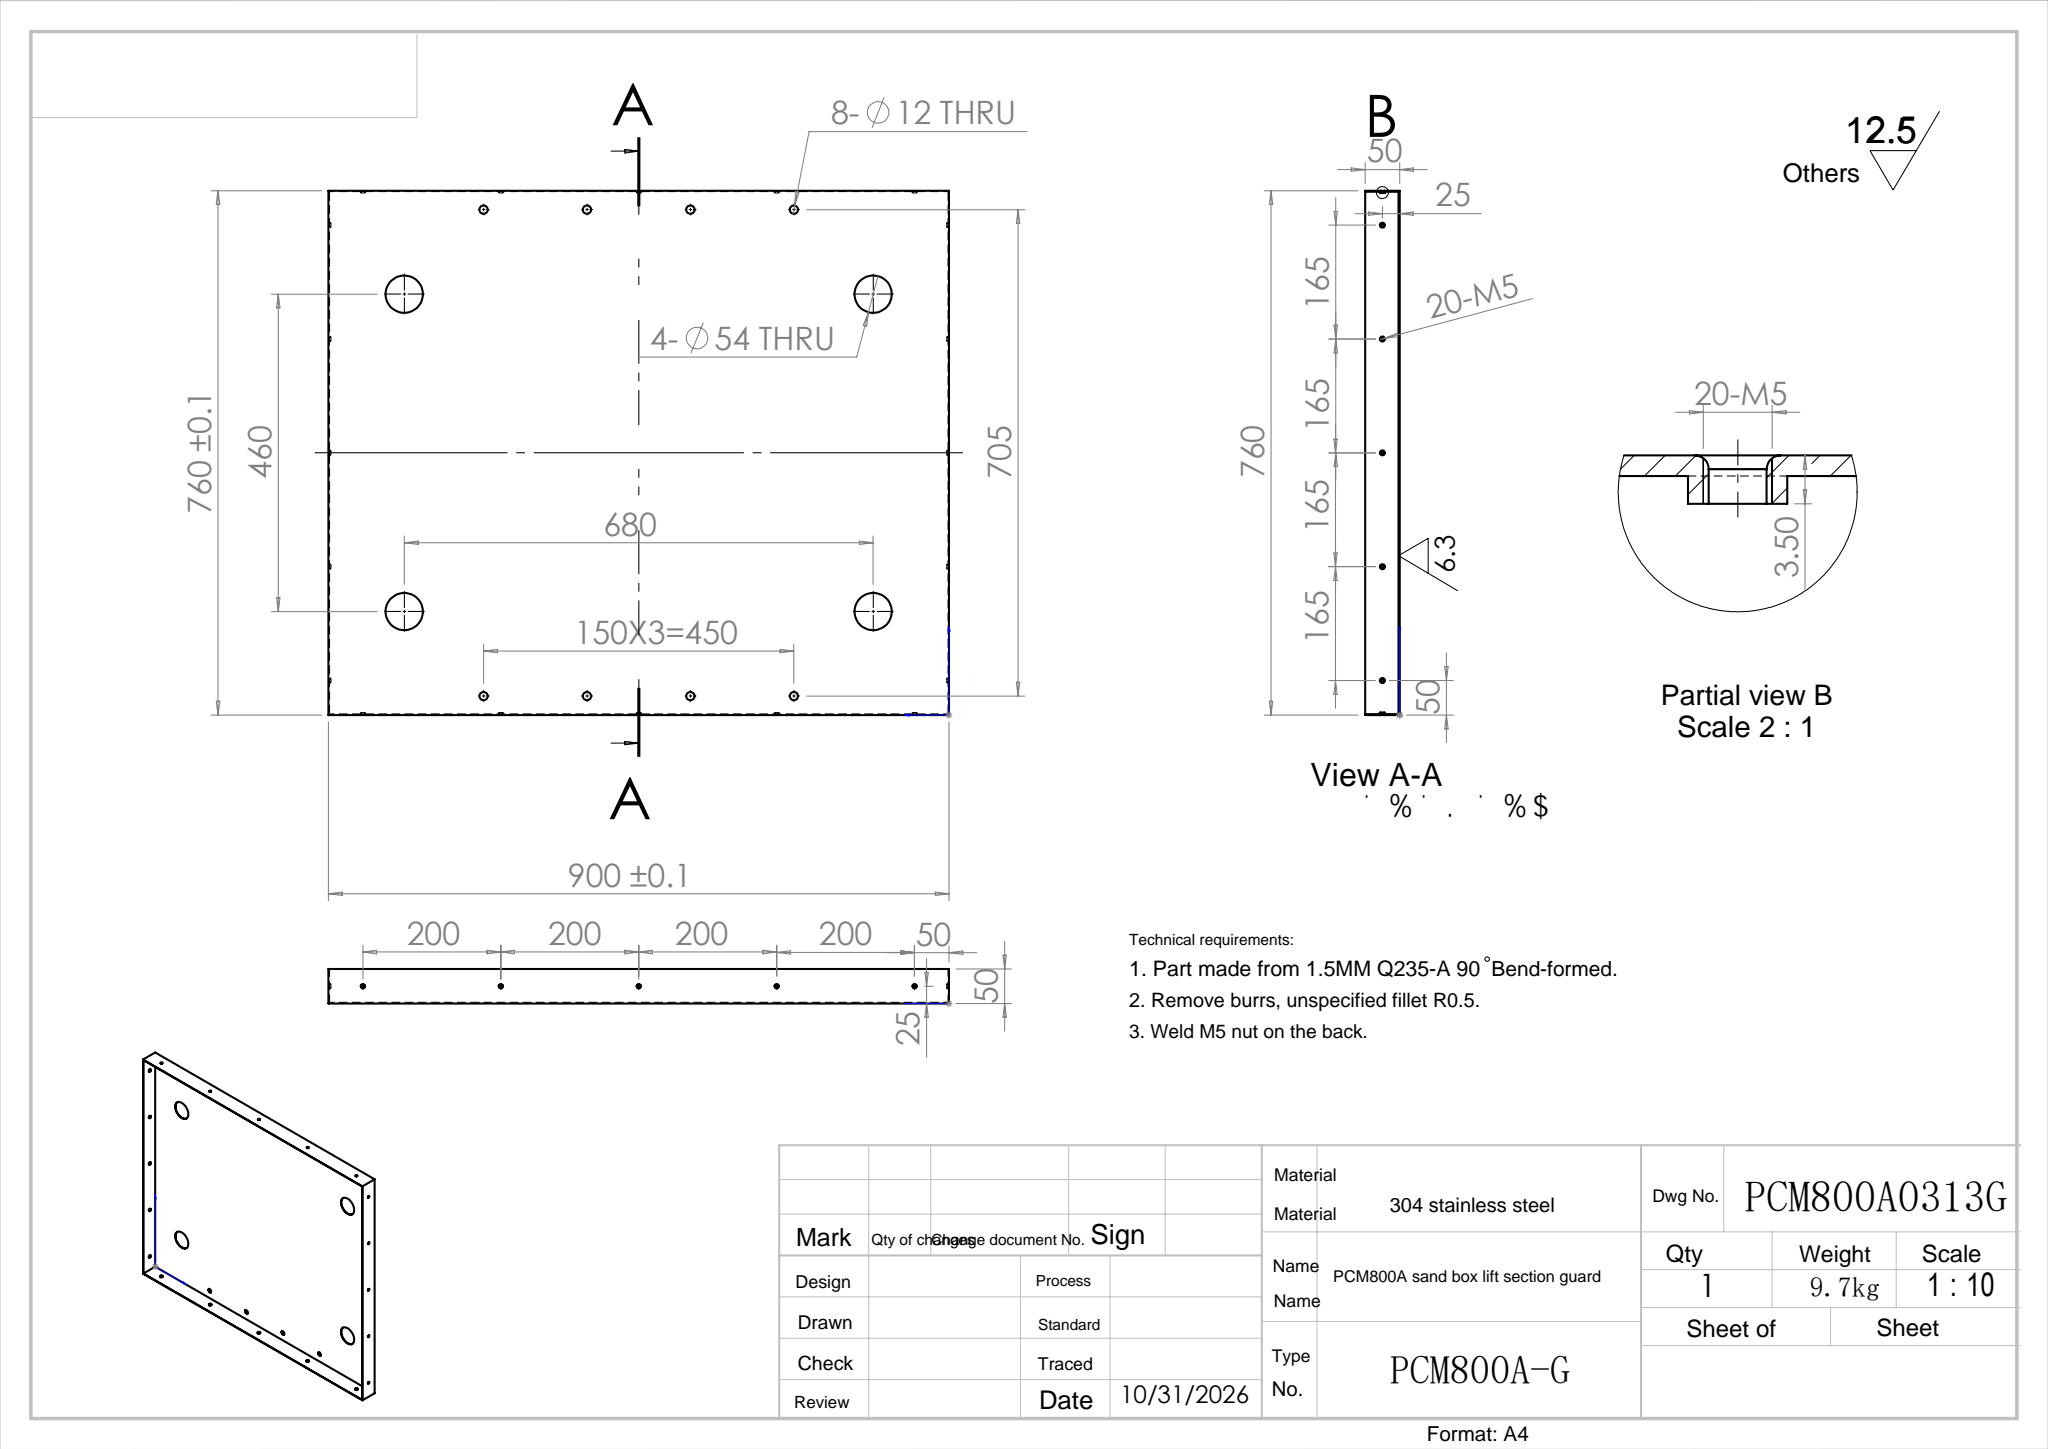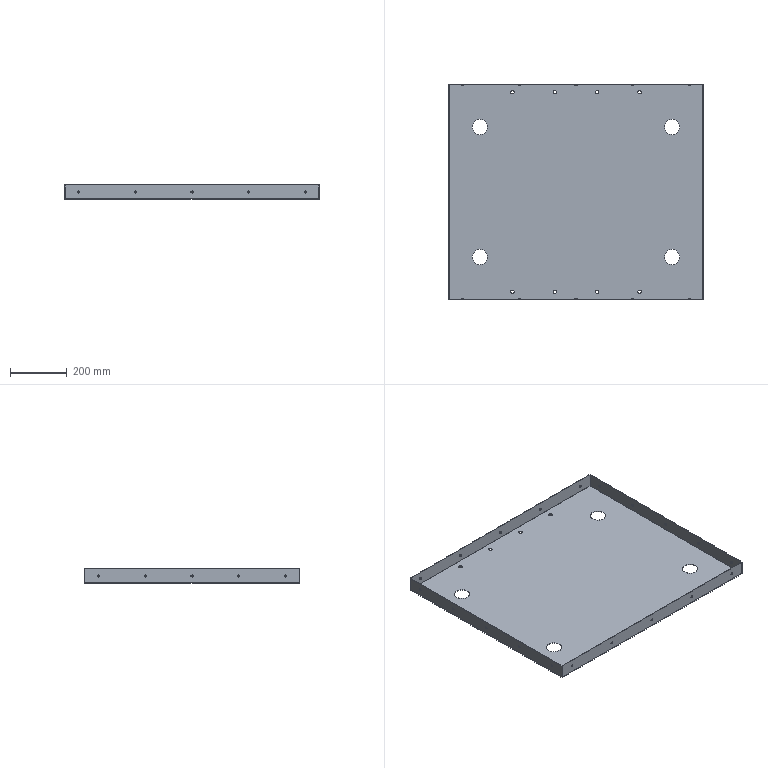Part | SolidWorks | features ICE 4, Cut 2, HoleWzd 2, Extrusion 1, Fillet 1, MirrorPattern 1, Shell 1 | 1 solid | 175 faces | box 900 x 760 x 50 mm | volume 1252591 mm3 | cylinder 104 | torus 40 | plane 31 | commonest cylinder face diameters 4.2 x40 7.2 x40 12 x16 54 x8